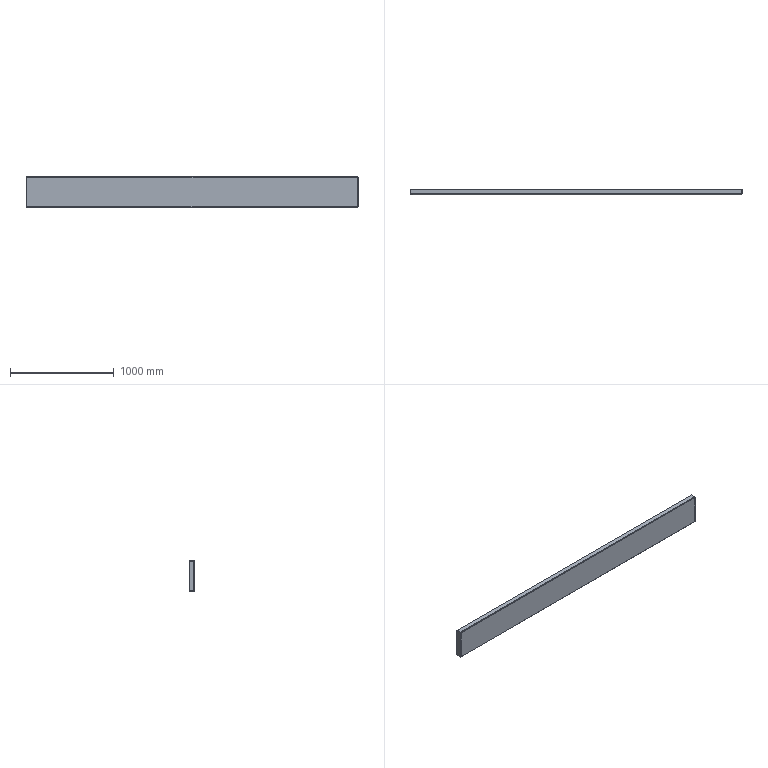Part | SolidWorks | features EdgeFlange 1, FlatPattern 1, SMBaseFlange 1, SheetMetal 1 | 1 solid | 38 faces | box 3200 x 50 x 294 mm | volume 3763315 mm3 | plane 22 | spline 8 | cylinder 8 | commonest cylinder face diameters 6 x4 12 x4